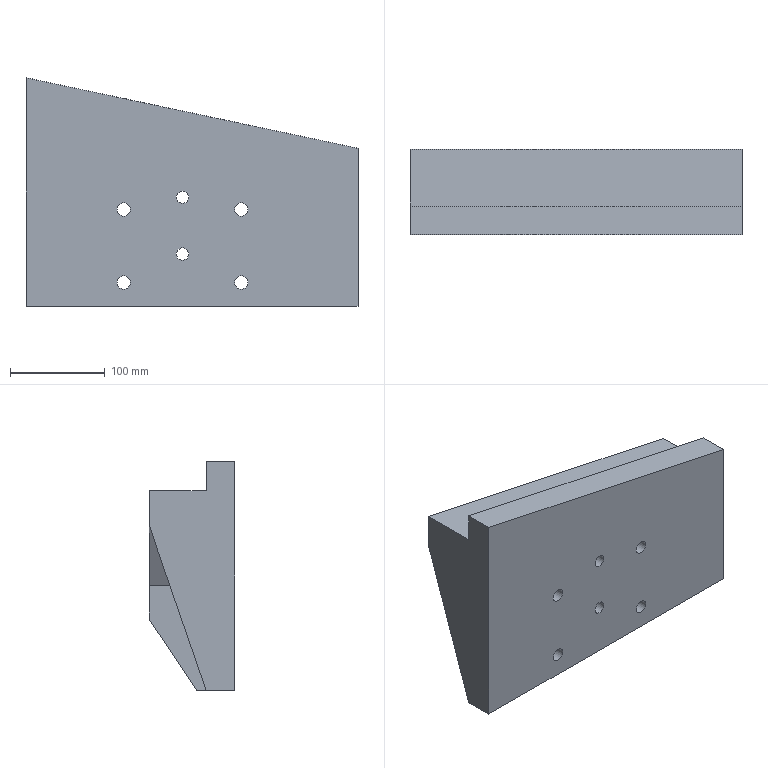Part | NX | features solid 2 | 1 solid | 28 faces | box 350 x 90 x 240.969 mm | volume 3053281 mm3 | plane 18 | cylinder 10 | commonest cylinder face diameters 14 x4 20 x4 13 x2
STEP:
#1=CARTESIAN_POINT('',(-565.,-580.,-83.));
#2=VERTEX_POINT('',#1);
#3=CARTESIAN_POINT('',(-572.,-580.,-83.));
#4=DIRECTION('',(0.,-1.,0.));
#5=DIRECTION('',(1.,0.,0.));
#6=AXIS2_PLACEMENT_3D('',#3,#4,#5);
#7=CIRCLE('',#6,7.);
#8=EDGE_CURVE('',#2,#2,#7,.T.);
#9=ORIENTED_EDGE('',*,*,#8,.T.);
#10=EDGE_LOOP('',(#9));
#11=FACE_BOUND('',#10,.T.);
#12=CARTESIAN_POINT('',(-562.,-580.,-83.));
#13=VERTEX_POINT('',#12);
#14=CARTESIAN_POINT('',(-572.,-580.,-83.));
#15=DIRECTION('',(0.,-1.,0.));
#16=DIRECTION('',(1.,0.,0.));
#17=AXIS2_PLACEMENT_3D('',#14,#15,#16);
#18=CIRCLE('',#17,10.);
#19=EDGE_CURVE('',#13,#13,#18,.T.);
#20=ORIENTED_EDGE('',*,*,#19,.F.);
#21=EDGE_LOOP('',(#20));
#22=FACE_BOUND('',#21,.T.);
#23=CARTESIAN_POINT('',(-572.,-580.,-83.));
#24=DIRECTION('',(0.,-1.,0.));
#25=DIRECTION('',(1.,0.,0.));
#26=AXIS2_PLACEMENT_3D('',#23,#24,#25);
#27=PLANE('',#26);
#28=ADVANCED_FACE('',(#11,#22),#27,.F.);
#29=CARTESIAN_POINT('',(-565.,-580.,-160.));
#30=VERTEX_POINT('',#29);
#31=CARTESIAN_POINT('',(-572.,-580.,-160.));
#32=DIRECTION('',(0.,-1.,0.));
#33=DIRECTION('',(1.,0.,0.));
#34=AXIS2_PLACEMENT_3D('',#31,#32,#33);
#35=CIRCLE('',#34,7.);
#36=EDGE_CURVE('',#30,#30,#35,.T.);
#37=ORIENTED_EDGE('',*,*,#36,.T.);
#38=EDGE_LOOP('',(#37));
#39=FACE_BOUND('',#38,.T.);
#40=CARTESIAN_POINT('',(-562.,-580.,-160.));
#41=VERTEX_POINT('',#40);
#42=CARTESIAN_POINT('',(-572.,-580.,-160.));
#43=DIRECTION('',(0.,-1.,0.));
#44=DIRECTION('',(1.,0.,0.));
#45=AXIS2_PLACEMENT_3D('',#42,#43,#44);
#46=CIRCLE('',#45,10.);
#47=EDGE_CURVE('',#41,#41,#46,.T.);
#48=ORIENTED_EDGE('',*,*,#47,.F.);
#49=EDGE_LOOP('',(#48));
#50=FACE_BOUND('',#49,.T.);
#51=CARTESIAN_POINT('',(-572.,-580.,-160.));
#52=DIRECTION('',(0.,-1.,0.));
#53=DIRECTION('',(1.,0.,0.));
#54=AXIS2_PLACEMENT_3D('',#51,#52,#53);
#55=PLANE('',#54);
#56=ADVANCED_FACE('',(#39,#50),#55,.F.);
#57=CARTESIAN_POINT('',(-441.,-580.,-160.));
#58=VERTEX_POINT('',#57);
#59=CARTESIAN_POINT('',(-448.,-580.,-160.));
#60=DIRECTION('',(0.,-1.,0.));
#61=DIRECTION('',(1.,0.,0.));
#62=AXIS2_PLACEMENT_3D('',#59,#60,#61);
#63=CIRCLE('',#62,7.);
#64=EDGE_CURVE('',#58,#58,#63,.T.);
#65=ORIENTED_EDGE('',*,*,#64,.T.);
#66=EDGE_LOOP('',(#65));
#67=FACE_BOUND('',#66,.T.);
#68=CARTESIAN_POINT('',(-438.,-580.,-160.));
#69=VERTEX_POINT('',#68);
#70=CARTESIAN_POINT('',(-448.,-580.,-160.));
#71=DIRECTION('',(0.,-1.,0.));
#72=DIRECTION('',(1.,0.,0.));
#73=AXIS2_PLACEMENT_3D('',#70,#71,#72);
#74=CIRCLE('',#73,10.);
#75=EDGE_CURVE('',#69,#69,#74,.T.);
#76=ORIENTED_EDGE('',*,*,#75,.F.);
#77=EDGE_LOOP('',(#76));
#78=FACE_BOUND('',#77,.T.);
#79=CARTESIAN_POINT('',(-448.,-580.,-160.));
#80=DIRECTION('',(0.,-1.,0.));
#81=DIRECTION('',(1.,0.,0.));
#82=AXIS2_PLACEMENT_3D('',#79,#80,#81);
#83=PLANE('',#82);
#84=ADVANCED_FACE('',(#67,#78),#83,.F.);
#85=CARTESIAN_POINT('',(-441.,-580.,-83.));
#86=VERTEX_POINT('',#85);
#87=CARTESIAN_POINT('',(-448.,-580.,-83.));
#88=DIRECTION('',(0.,-1.,0.));
#89=DIRECTION('',(1.,0.,0.));
#90=AXIS2_PLACEMENT_3D('',#87,#88,#89);
#91=CIRCLE('',#90,7.);
#92=EDGE_CURVE('',#86,#86,#91,.T.);
#93=ORIENTED_EDGE('',*,*,#92,.T.);
#94=EDGE_LOOP('',(#93));
#95=FACE_BOUND('',#94,.T.);
#96=CARTESIAN_POINT('',(-438.,-580.,-83.));
#97=VERTEX_POINT('',#96);
#98=CARTESIAN_POINT('',(-448.,-580.,-83.));
#99=DIRECTION('',(0.,-1.,0.));
#100=DIRECTION('',(1.,0.,0.));
#101=AXIS2_PLACEMENT_3D('',#98,#99,#100);
#102=CIRCLE('',#101,10.);
#103=EDGE_CURVE('',#97,#97,#102,.T.);
#104=ORIENTED_EDGE('',*,*,#103,.F.);
#105=EDGE_LOOP('',(#104));
#106=FACE_BOUND('',#105,.T.);
#107=CARTESIAN_POINT('',(-448.,-580.,-83.));
#108=DIRECTION('',(0.,-1.,0.));
#109=DIRECTION('',(1.,0.,0.));
#110=AXIS2_PLACEMENT_3D('',#107,#108,#109);
#111=PLANE('',#110);
#112=ADVANCED_FACE('',(#95,#106),#111,.F.);
#113=CARTESIAN_POINT('',(-640.,-570.,-12.811));
#114=VERTEX_POINT('',#113);
#115=CARTESIAN_POINT('',(-640.,-570.,-185.));
#116=VERTEX_POINT('',#115);
#117=CARTESIAN_POINT('',(-640.,-570.,-55.974));
#118=DIRECTION('',(0.,0.,-1.));
#119=VECTOR('',#118,1000.);
#120=LINE('',#117,#119);
#121=EDGE_CURVE('',#114,#116,#120,.T.);
#122=ORIENTED_EDGE('',*,*,#121,.T.);
#123=CARTESIAN_POINT('',(-640.,-510.368,-12.811));
#124=VERTEX_POINT('',#123);
#125=CARTESIAN_POINT('',(-640.,-551.446,-131.426));
#126=DIRECTION('',(0.,0.3272,0.9449));
#127=VECTOR('',#126,1000.);
#128=LINE('',#125,#127);
#129=EDGE_CURVE('',#116,#124,#128,.T.);
#130=ORIENTED_EDGE('',*,*,#129,.T.);
#131=CARTESIAN_POINT('',(-640.,-570.,-12.811));
#132=DIRECTION('',(0.,1.,0.));
#133=VECTOR('',#132,1000.);
#134=LINE('',#131,#133);
#135=EDGE_CURVE('',#114,#124,#134,.T.);
#136=ORIENTED_EDGE('',*,*,#135,.F.);
#137=EDGE_LOOP('',(#122,#130,#136));
#138=FACE_BOUND('',#137,.T.);
#139=CARTESIAN_POINT('',(-640.,-570.,-125.));
#140=DIRECTION('',(-1.,0.,0.));
#141=DIRECTION('',(0.,0.,-1.));
#142=AXIS2_PLACEMENT_3D('',#139,#140,#141);
#143=PLANE('',#142);
#144=ADVANCED_FACE('',(#138),#143,.F.);
#145=ORIENTED_EDGE('',*,*,#47,.T.);
#146=EDGE_LOOP('',(#145));
#147=FACE_BOUND('',#146,.T.);
#148=CARTESIAN_POINT('',(-562.,-570.,-160.));
#149=VERTEX_POINT('',#148);
#150=CARTESIAN_POINT('',(-572.,-570.,-160.));
#151=DIRECTION('',(0.,-1.,0.));
#152=DIRECTION('',(1.,0.,0.));
#153=AXIS2_PLACEMENT_3D('',#150,#151,#152);
#154=CIRCLE('',#153,10.);
#155=EDGE_CURVE('',#149,#149,#154,.T.);
#156=ORIENTED_EDGE('',*,*,#155,.F.);
#157=EDGE_LOOP('',(#156));
#158=FACE_BOUND('',#157,.T.);
#159=CARTESIAN_POINT('',(-572.,-570.,-160.));
#160=DIRECTION('',(0.,-1.,0.));
#161=DIRECTION('',(1.,0.,0.));
#162=AXIS2_PLACEMENT_3D('',#159,#160,#161);
#163=CYLINDRICAL_SURFACE('',#162,10.);
#164=ADVANCED_FACE('',(#147,#158),#163,.F.);
#165=ORIENTED_EDGE('',*,*,#75,.T.);
#166=EDGE_LOOP('',(#165));
#167=FACE_BOUND('',#166,.T.);
#168=CARTESIAN_POINT('',(-438.,-570.,-160.));
#169=VERTEX_POINT('',#168);
#170=CARTESIAN_POINT('',(-448.,-570.,-160.));
#171=DIRECTION('',(0.,-1.,0.));
#172=DIRECTION('',(1.,0.,0.));
#173=AXIS2_PLACEMENT_3D('',#170,#171,#172);
#174=CIRCLE('',#173,10.);
#175=EDGE_CURVE('',#169,#169,#174,.T.);
#176=ORIENTED_EDGE('',*,*,#175,.F.);
#177=EDGE_LOOP('',(#176));
#178=FACE_BOUND('',#177,.T.);
#179=CARTESIAN_POINT('',(-448.,-570.,-160.));
#180=DIRECTION('',(0.,-1.,0.));
#181=DIRECTION('',(1.,0.,0.));
#182=AXIS2_PLACEMENT_3D('',#179,#180,#181);
#183=CYLINDRICAL_SURFACE('',#182,10.);
#184=ADVANCED_FACE('',(#167,#178),#183,.F.);
#185=ORIENTED_EDGE('',*,*,#19,.T.);
#186=EDGE_LOOP('',(#185));
#187=FACE_BOUND('',#186,.T.);
#188=CARTESIAN_POINT('',(-562.,-570.,-83.));
#189=VERTEX_POINT('',#188);
#190=CARTESIAN_POINT('',(-572.,-570.,-83.));
#191=DIRECTION('',(0.,-1.,0.));
#192=DIRECTION('',(1.,0.,0.));
#193=AXIS2_PLACEMENT_3D('',#190,#191,#192);
#194=CIRCLE('',#193,10.);
#195=EDGE_CURVE('',#189,#189,#194,.T.);
#196=ORIENTED_EDGE('',*,*,#195,.F.);
#197=EDGE_LOOP('',(#196));
#198=FACE_BOUND('',#197,.T.);
#199=CARTESIAN_POINT('',(-572.,-570.,-83.));
#200=DIRECTION('',(0.,-1.,0.));
#201=DIRECTION('',(1.,0.,0.));
#202=AXIS2_PLACEMENT_3D('',#199,#200,#201);
#203=CYLINDRICAL_SURFACE('',#202,10.);
#204=ADVANCED_FACE('',(#187,#198),#203,.F.);
#205=ORIENTED_EDGE('',*,*,#103,.T.);
#206=EDGE_LOOP('',(#205));
#207=FACE_BOUND('',#206,.T.);
#208=CARTESIAN_POINT('',(-438.,-570.,-83.));
#209=VERTEX_POINT('',#208);
#210=CARTESIAN_POINT('',(-448.,-570.,-83.));
#211=DIRECTION('',(0.,-1.,0.));
#212=DIRECTION('',(1.,0.,0.));
#213=AXIS2_PLACEMENT_3D('',#210,#211,#212);
#214=CIRCLE('',#213,10.);
#215=EDGE_CURVE('',#209,#209,#214,.T.);
#216=ORIENTED_EDGE('',*,*,#215,.F.);
#217=EDGE_LOOP('',(#216));
#218=FACE_BOUND('',#217,.T.);
#219=CARTESIAN_POINT('',(-448.,-570.,-83.));
#220=DIRECTION('',(0.,-1.,0.));
#221=DIRECTION('',(1.,0.,0.));
#222=AXIS2_PLACEMENT_3D('',#219,#220,#221);
#223=CYLINDRICAL_SURFACE('',#222,10.);
#224=ADVANCED_FACE('',(#207,#218),#223,.F.);
#225=ORIENTED_EDGE('',*,*,#8,.F.);
#226=EDGE_LOOP('',(#225));
#227=FACE_BOUND('',#226,.T.);
#228=CARTESIAN_POINT('',(-565.,-600.,-83.));
#229=VERTEX_POINT('',#228);
#230=CARTESIAN_POINT('',(-572.,-600.,-83.));
#231=DIRECTION('',(0.,-1.,0.));
#232=DIRECTION('',(1.,0.,0.));
#233=AXIS2_PLACEMENT_3D('',#230,#231,#232);
#234=CIRCLE('',#233,7.);
#235=EDGE_CURVE('',#229,#229,#234,.F.);
#236=ORIENTED_EDGE('',*,*,#235,.F.);
#237=EDGE_LOOP('',(#236));
#238=FACE_BOUND('',#237,.T.);
#239=CARTESIAN_POINT('',(-572.,-700.,-83.));
#240=DIRECTION('',(0.,1.,0.));
#241=DIRECTION('',(0.,0.,-1.));
#242=AXIS2_PLACEMENT_3D('',#239,#240,#241);
#243=CYLINDRICAL_SURFACE('',#242,7.);
#244=ADVANCED_FACE('',(#227,#238),#243,.F.);
#245=CARTESIAN_POINT('',(-503.5,-600.,-70.));
#246=VERTEX_POINT('',#245);
#247=CARTESIAN_POINT('',(-510.,-600.,-70.));
#248=DIRECTION('',(0.,-1.,0.));
#249=DIRECTION('',(1.,0.,0.));
#250=AXIS2_PLACEMENT_3D('',#247,#248,#249);
#251=CIRCLE('',#250,6.5);
#252=EDGE_CURVE('',#246,#246,#251,.T.);
#253=ORIENTED_EDGE('',*,*,#252,.T.);
#254=EDGE_LOOP('',(#253));
#255=FACE_BOUND('',#254,.T.);
#256=CARTESIAN_POINT('',(-503.5,-570.,-70.));
#257=VERTEX_POINT('',#256);
#258=CARTESIAN_POINT('',(-510.,-570.,-70.));
#259=DIRECTION('',(0.,-1.,0.));
#260=DIRECTION('',(1.,0.,0.));
#261=AXIS2_PLACEMENT_3D('',#258,#259,#260);
#262=CIRCLE('',#261,6.5);
#263=EDGE_CURVE('',#257,#257,#262,.T.);
#264=ORIENTED_EDGE('',*,*,#263,.F.);
#265=EDGE_LOOP('',(#264));
#266=FACE_BOUND('',#265,.T.);
#267=CARTESIAN_POINT('',(-510.,-700.,-70.));
#268=DIRECTION('',(0.,1.,0.));
#269=DIRECTION('',(0.,0.,-1.));
#270=AXIS2_PLACEMENT_3D('',#267,#268,#269);
#271=CYLINDRICAL_SURFACE('',#270,6.5);
#272=ADVANCED_FACE('',(#255,#266),#271,.F.);
#273=ORIENTED_EDGE('',*,*,#36,.F.);
#274=EDGE_LOOP('',(#273));
#275=FACE_BOUND('',#274,.T.);
#276=CARTESIAN_POINT('',(-565.,-600.,-160.));
#277=VERTEX_POINT('',#276);
#278=CARTESIAN_POINT('',(-572.,-600.,-160.));
#279=DIRECTION('',(0.,-1.,0.));
#280=DIRECTION('',(1.,0.,0.));
#281=AXIS2_PLACEMENT_3D('',#278,#279,#280);
#282=CIRCLE('',#281,7.);
#283=EDGE_CURVE('',#277,#277,#282,.F.);
#284=ORIENTED_EDGE('',*,*,#283,.F.);
#285=EDGE_LOOP('',(#284));
#286=FACE_BOUND('',#285,.T.);
#287=CARTESIAN_POINT('',(-572.,-700.,-160.));
#288=DIRECTION('',(0.,1.,0.));
#289=DIRECTION('',(0.,0.,-1.));
#290=AXIS2_PLACEMENT_3D('',#287,#288,#289);
#291=CYLINDRICAL_SURFACE('',#290,7.);
#292=ADVANCED_FACE('',(#275,#286),#291,.F.);
#293=CARTESIAN_POINT('',(-503.5,-600.,-130.));
#294=VERTEX_POINT('',#293);
#295=CARTESIAN_POINT('',(-510.,-600.,-130.));
#296=DIRECTION('',(0.,-1.,0.));
#297=DIRECTION('',(1.,0.,0.));
#298=AXIS2_PLACEMENT_3D('',#295,#296,#297);
#299=CIRCLE('',#298,6.5);
#300=EDGE_CURVE('',#294,#294,#299,.T.);
#301=ORIENTED_EDGE('',*,*,#300,.T.);
#302=EDGE_LOOP('',(#301));
#303=FACE_BOUND('',#302,.T.);
#304=CARTESIAN_POINT('',(-503.5,-570.,-130.));
#305=VERTEX_POINT('',#304);
#306=CARTESIAN_POINT('',(-510.,-570.,-130.));
#307=DIRECTION('',(0.,-1.,0.));
#308=DIRECTION('',(1.,0.,0.));
#309=AXIS2_PLACEMENT_3D('',#306,#307,#308);
#310=CIRCLE('',#309,6.5);
#311=EDGE_CURVE('',#305,#305,#310,.T.);
#312=ORIENTED_EDGE('',*,*,#311,.F.);
#313=EDGE_LOOP('',(#312));
#314=FACE_BOUND('',#313,.T.);
#315=CARTESIAN_POINT('',(-510.,-700.,-130.));
#316=DIRECTION('',(0.,1.,0.));
#317=DIRECTION('',(0.,0.,-1.));
#318=AXIS2_PLACEMENT_3D('',#315,#316,#317);
#319=CYLINDRICAL_SURFACE('',#318,6.5);
#320=ADVANCED_FACE('',(#303,#314),#319,.F.);
#321=ORIENTED_EDGE('',*,*,#64,.F.);
#322=EDGE_LOOP('',(#321));
#323=FACE_BOUND('',#322,.T.);
#324=CARTESIAN_POINT('',(-441.,-600.,-160.));
#325=VERTEX_POINT('',#324);
#326=CARTESIAN_POINT('',(-448.,-600.,-160.));
#327=DIRECTION('',(0.,-1.,0.));
#328=DIRECTION('',(1.,0.,0.));
#329=AXIS2_PLACEMENT_3D('',#326,#327,#328);
#330=CIRCLE('',#329,7.);
#331=EDGE_CURVE('',#325,#325,#330,.F.);
#332=ORIENTED_EDGE('',*,*,#331,.F.);
#333=EDGE_LOOP('',(#332));
#334=FACE_BOUND('',#333,.T.);
#335=CARTESIAN_POINT('',(-448.,-700.,-160.));
#336=DIRECTION('',(0.,1.,0.));
#337=DIRECTION('',(0.,0.,-1.));
#338=AXIS2_PLACEMENT_3D('',#335,#336,#337);
#339=CYLINDRICAL_SURFACE('',#338,7.);
#340=ADVANCED_FACE('',(#323,#334),#339,.F.);
#341=ORIENTED_EDGE('',*,*,#92,.F.);
#342=EDGE_LOOP('',(#341));
#343=FACE_BOUND('',#342,.T.);
#344=CARTESIAN_POINT('',(-441.,-600.,-83.));
#345=VERTEX_POINT('',#344);
#346=CARTESIAN_POINT('',(-448.,-600.,-83.));
#347=DIRECTION('',(0.,-1.,0.));
#348=DIRECTION('',(1.,0.,0.));
#349=AXIS2_PLACEMENT_3D('',#346,#347,#348);
#350=CIRCLE('',#349,7.);
#351=EDGE_CURVE('',#345,#345,#350,.F.);
#352=ORIENTED_EDGE('',*,*,#351,.F.);
#353=EDGE_LOOP('',(#352));
#354=FACE_BOUND('',#353,.T.);
#355=CARTESIAN_POINT('',(-448.,-700.,-83.));
#356=DIRECTION('',(0.,1.,0.));
#357=DIRECTION('',(0.,0.,-1.));
#358=AXIS2_PLACEMENT_3D('',#355,#356,#357);
#359=CYLINDRICAL_SURFACE('',#358,7.);
#360=ADVANCED_FACE('',(#343,#354),#359,.F.);
#361=CARTESIAN_POINT('',(-675.,-600.,-185.));
#362=VERTEX_POINT('',#361);
#363=CARTESIAN_POINT('',(-675.,-570.,-185.));
#364=VERTEX_POINT('',#363);
#365=CARTESIAN_POINT('',(-675.,-600.,-185.));
#366=DIRECTION('',(0.,1.,0.));
#367=VECTOR('',#366,1000.);
#368=LINE('',#365,#367);
#369=EDGE_CURVE('',#362,#364,#368,.T.);
#370=ORIENTED_EDGE('',*,*,#369,.T.);
#371=CARTESIAN_POINT('',(-305.,-570.,-185.));
#372=DIRECTION('',(-1.,0.,0.));
#373=VECTOR('',#372,1000.);
#374=LINE('',#371,#373);
#375=EDGE_CURVE('',#116,#364,#374,.T.);
#376=ORIENTED_EDGE('',*,*,#375,.F.);
#377=CARTESIAN_POINT('',(-350.,-570.,-185.));
#378=VERTEX_POINT('',#377);
#379=CARTESIAN_POINT('',(-695.,-570.,-185.));
#380=DIRECTION('',(1.,0.,0.));
#381=VECTOR('',#380,1000.);
#382=LINE('',#379,#381);
#383=EDGE_CURVE('',#378,#116,#382,.F.);
#384=ORIENTED_EDGE('',*,*,#383,.F.);
#385=CARTESIAN_POINT('',(-350.,-560.,-185.));
#386=VERTEX_POINT('',#385);
#387=CARTESIAN_POINT('',(-350.,-570.,-185.));
#388=DIRECTION('',(0.,1.,0.));
#389=VECTOR('',#388,1000.);
#390=LINE('',#387,#389);
#391=EDGE_CURVE('',#386,#378,#390,.F.);
#392=ORIENTED_EDGE('',*,*,#391,.F.);
#393=CARTESIAN_POINT('',(-325.,-560.,-185.));
#394=VERTEX_POINT('',#393);
#395=CARTESIAN_POINT('',(-270.,-560.,-185.));
#396=DIRECTION('',(1.,0.,0.));
#397=VECTOR('',#396,1000.);
#398=LINE('',#395,#397);
#399=EDGE_CURVE('',#386,#394,#398,.T.);
#400=ORIENTED_EDGE('',*,*,#399,.T.);
#401=CARTESIAN_POINT('',(-325.,-600.,-185.));
#402=VERTEX_POINT('',#401);
#403=CARTESIAN_POINT('',(-325.,-515.,-185.));
#404=DIRECTION('',(0.,-1.,0.));
#405=VECTOR('',#404,1000.);
#406=LINE('',#403,#405);
#407=EDGE_CURVE('',#402,#394,#406,.F.);
#408=ORIENTED_EDGE('',*,*,#407,.F.);
#409=CARTESIAN_POINT('',(275.,-600.,-185.));
#410=DIRECTION('',(1.,0.,0.));
#411=VECTOR('',#410,1000.);
#412=LINE('',#409,#411);
#413=EDGE_CURVE('',#402,#362,#412,.F.);
#414=ORIENTED_EDGE('',*,*,#413,.T.);
#415=EDGE_LOOP('',(#370,#376,#384,#392,#400,#408,#414));
#416=FACE_BOUND('',#415,.T.);
#417=CARTESIAN_POINT('',(460.,-600.,-185.));
#418=DIRECTION('',(0.,0.,-1.));
#419=DIRECTION('',(0.,-1.,0.));
#420=AXIS2_PLACEMENT_3D('',#417,#418,#419);
#421=PLANE('',#420);
#422=ADVANCED_FACE('',(#416),#421,.T.);
#423=CARTESIAN_POINT('',(-675.,-570.,25.298));
#424=VERTEX_POINT('',#423);
#425=CARTESIAN_POINT('',(-675.,-570.,55.969));
#426=VERTEX_POINT('',#425);
#427=CARTESIAN_POINT('',(-675.,-570.,-55.974));
#428=DIRECTION('',(0.,0.,1.));
#429=VECTOR('',#428,1000.);
#430=LINE('',#427,#429);
#431=EDGE_CURVE('',#424,#426,#430,.T.);
#432=ORIENTED_EDGE('',*,*,#431,.F.);
#433=CARTESIAN_POINT('',(-675.,-510.,25.298));
#434=VERTEX_POINT('',#433);
#435=CARTESIAN_POINT('',(-675.,-5.,25.298));
#436=DIRECTION('',(0.,-1.,0.));
#437=VECTOR('',#436,1000.);
#438=LINE('',#435,#437);
#439=EDGE_CURVE('',#434,#424,#438,.T.);
#440=ORIENTED_EDGE('',*,*,#439,.F.);
#441=CARTESIAN_POINT('',(-675.,-510.,-11.749));
#442=VERTEX_POINT('',#441);
#443=CARTESIAN_POINT('',(-675.,-510.,-95.974));
#444=DIRECTION('',(0.,0.,-1.));
#445=VECTOR('',#444,1000.);
#446=LINE('',#443,#445);
#447=EDGE_CURVE('',#442,#434,#446,.F.);
#448=ORIENTED_EDGE('',*,*,#447,.F.);
#449=CARTESIAN_POINT('',(-675.,-452.286,154.903));
#450=DIRECTION('',(0.,0.3272,0.9449));
#451=VECTOR('',#450,1000.);
#452=LINE('',#449,#451);
#453=EDGE_CURVE('',#442,#364,#452,.F.);
#454=ORIENTED_EDGE('',*,*,#453,.T.);
#455=ORIENTED_EDGE('',*,*,#369,.F.);
#456=CARTESIAN_POINT('',(-675.,-600.,55.969));
#457=VERTEX_POINT('',#456);
#458=CARTESIAN_POINT('',(-675.,-600.,-55.974));
#459=DIRECTION('',(0.,0.,1.));
#460=VECTOR('',#459,1000.);
#461=LINE('',#458,#460);
#462=EDGE_CURVE('',#362,#457,#461,.T.);
#463=ORIENTED_EDGE('',*,*,#462,.T.);
#464=CARTESIAN_POINT('',(-675.,-5.,55.969));
#465=DIRECTION('',(0.,-1.,0.));
#466=VECTOR('',#465,1000.);
#467=LINE('',#464,#466);
#468=EDGE_CURVE('',#426,#457,#467,.T.);
#469=ORIENTED_EDGE('',*,*,#468,.F.);
#470=EDGE_LOOP('',(#432,#440,#448,#454,#455,#463,#469));
#471=FACE_BOUND('',#470,.T.);
#472=CARTESIAN_POINT('',(-675.,-5.,0.));
#473=DIRECTION('',(-1.,0.,0.));
#474=DIRECTION('',(0.,0.,-1.));
#475=AXIS2_PLACEMENT_3D('',#472,#473,#474);
#476=PLANE('',#475);
#477=ADVANCED_FACE('',(#471),#476,.T.);
#478=ORIENTED_EDGE('',*,*,#375,.T.);
#479=ORIENTED_EDGE('',*,*,#453,.F.);
#480=CARTESIAN_POINT('',(-645.,-510.,-11.749));
#481=VERTEX_POINT('',#480);
#482=CARTESIAN_POINT('',(-595.,-510.,-11.749));
#483=DIRECTION('',(-1.,0.,0.));
#484=VECTOR('',#483,1000.);
#485=LINE('',#482,#484);
#486=EDGE_CURVE('',#481,#442,#485,.T.);
#487=ORIENTED_EDGE('',*,*,#486,.F.);
#488=CARTESIAN_POINT('',(-558.152,-516.393,-30.209));
#489=DIRECTION('',(-0.9756,0.07182,0.2074));
#490=VECTOR('',#489,1000.);
#491=LINE('',#488,#490);
#492=EDGE_CURVE('',#124,#481,#491,.T.);
#493=ORIENTED_EDGE('',*,*,#492,.F.);
#494=ORIENTED_EDGE('',*,*,#129,.F.);
#495=EDGE_LOOP('',(#478,#479,#487,#493,#494));
#496=FACE_BOUND('',#495,.T.);
#497=CARTESIAN_POINT('',(-595.,-570.,-185.));
#498=DIRECTION('',(0.,-0.9449,0.3272));
#499=DIRECTION('',(0.,-0.3272,-0.9449));
#500=AXIS2_PLACEMENT_3D('',#497,#498,#499);
#501=PLANE('',#500);
#502=ADVANCED_FACE('',(#496),#501,.F.);
#503=ORIENTED_EDGE('',*,*,#135,.T.);
#504=ORIENTED_EDGE('',*,*,#492,.T.);
#505=CARTESIAN_POINT('',(-350.,-510.,-74.453));
#506=VERTEX_POINT('',#505);
#507=CARTESIAN_POINT('',(252.36,-510.,-202.488));
#508=DIRECTION('',(-0.9781,0.,0.2079));
#509=VECTOR('',#508,1000.);
#510=LINE('',#507,#509);
#511=EDGE_CURVE('',#506,#481,#510,.T.);
#512=ORIENTED_EDGE('',*,*,#511,.F.);
#513=CARTESIAN_POINT('',(-350.,-570.,-74.453));
#514=VERTEX_POINT('',#513);
#515=CARTESIAN_POINT('',(-350.,-570.,-74.453));
#516=DIRECTION('',(0.,-1.,0.));
#517=VECTOR('',#516,1000.);
#518=LINE('',#515,#517);
#519=EDGE_CURVE('',#514,#506,#518,.F.);
#520=ORIENTED_EDGE('',*,*,#519,.F.);
#521=CARTESIAN_POINT('',(-683.845,-570.,-3.492));
#522=DIRECTION('',(-0.9781,0.,0.2079));
#523=VECTOR('',#522,1000.);
#524=LINE('',#521,#523);
#525=EDGE_CURVE('',#514,#114,#524,.T.);
#526=ORIENTED_EDGE('',*,*,#525,.T.);
#527=EDGE_LOOP('',(#503,#504,#512,#520,#526));
#528=FACE_BOUND('',#527,.T.);
#529=CARTESIAN_POINT('',(-342.997,-570.,-75.941));
#530=DIRECTION('',(0.2079,0.,0.9781));
#531=DIRECTION('',(-0.9781,0.,0.2079));
#532=AXIS2_PLACEMENT_3D('',#529,#530,#531);
#533=PLANE('',#532);
#534=ADVANCED_FACE('',(#528),#533,.F.);
#535=CARTESIAN_POINT('',(-350.,-510.,-110.));
#536=VERTEX_POINT('',#535);
#537=CARTESIAN_POINT('',(-350.,-535.385,-148.077));
#538=DIRECTION('',(0.,-0.5547,-0.8321));
#539=VECTOR('',#538,1000.);
#540=LINE('',#537,#539);
#541=EDGE_CURVE('',#386,#536,#540,.F.);
#542=ORIENTED_EDGE('',*,*,#541,.F.);
#543=ORIENTED_EDGE('',*,*,#391,.T.);
#544=CARTESIAN_POINT('',(-350.,-570.,-125.));
#545=DIRECTION('',(0.,0.,1.));
#546=VECTOR('',#545,1000.);
#547=LINE('',#544,#546);
#548=EDGE_CURVE('',#514,#378,#547,.F.);
#549=ORIENTED_EDGE('',*,*,#548,.F.);
#550=ORIENTED_EDGE('',*,*,#519,.T.);
#551=CARTESIAN_POINT('',(-350.,-510.,-125.));
#552=DIRECTION('',(0.,0.,1.));
#553=VECTOR('',#552,1000.);
#554=LINE('',#551,#553);
#555=EDGE_CURVE('',#506,#536,#554,.F.);
#556=ORIENTED_EDGE('',*,*,#555,.T.);
#557=EDGE_LOOP('',(#542,#543,#549,#550,#556));
#558=FACE_BOUND('',#557,.T.);
#559=CARTESIAN_POINT('',(-350.,-570.,-125.));
#560=DIRECTION('',(-1.,0.,0.));
#561=DIRECTION('',(0.,0.,-1.));
#562=AXIS2_PLACEMENT_3D('',#559,#560,#561);
#563=PLANE('',#562);
#564=ADVANCED_FACE('',(#558),#563,.T.);
#565=CARTESIAN_POINT('',(-325.,-600.,-18.426));
#566=VERTEX_POINT('',#565);
#567=CARTESIAN_POINT('',(-325.,-600.,-55.974));
#568=DIRECTION('',(0.,0.,-1.));
#569=VECTOR('',#568,1000.);
#570=LINE('',#567,#569);
#571=EDGE_CURVE('',#566,#402,#570,.T.);
#572=ORIENTED_EDGE('',*,*,#571,.T.);
#573=ORIENTED_EDGE('',*,*,#407,.T.);
#574=CARTESIAN_POINT('',(-325.,-510.,-110.));
#575=VERTEX_POINT('',#574);
#576=CARTESIAN_POINT('',(-325.,-543.83,-160.745));
#577=DIRECTION('',(0.,0.5547,0.8321));
#578=VECTOR('',#577,1000.);
#579=LINE('',#576,#578);
#580=EDGE_CURVE('',#575,#394,#579,.F.);
#581=ORIENTED_EDGE('',*,*,#580,.F.);
#582=CARTESIAN_POINT('',(-325.,-510.,-49.096));
#583=VERTEX_POINT('',#582);
#584=CARTESIAN_POINT('',(-325.,-510.,-179.965));
#585=DIRECTION('',(0.,0.,-1.));
#586=VECTOR('',#585,1000.);
#587=LINE('',#584,#586);
#588=EDGE_CURVE('',#575,#583,#587,.F.);
#589=ORIENTED_EDGE('',*,*,#588,.T.);
#590=CARTESIAN_POINT('',(-325.,-570.,-49.096));
#591=VERTEX_POINT('',#590);
#592=CARTESIAN_POINT('',(-325.,-535.533,-49.096));
#593=DIRECTION('',(0.,-1.,0.));
#594=VECTOR('',#593,1000.);
#595=LINE('',#592,#594);
#596=EDGE_CURVE('',#583,#591,#595,.T.);
#597=ORIENTED_EDGE('',*,*,#596,.T.);
#598=CARTESIAN_POINT('',(-325.,-570.,-18.426));
#599=VERTEX_POINT('',#598);
#600=CARTESIAN_POINT('',(-325.,-570.,-90.));
#601=DIRECTION('',(0.,0.,1.));
#602=VECTOR('',#601,1000.);
#603=LINE('',#600,#602);
#604=EDGE_CURVE('',#591,#599,#603,.T.);
#605=ORIENTED_EDGE('',*,*,#604,.T.);
#606=CARTESIAN_POINT('',(-325.,-535.533,-18.426));
#607=DIRECTION('',(0.,-1.,0.));
#608=VECTOR('',#607,1000.);
#609=LINE('',#606,#608);
#610=EDGE_CURVE('',#599,#566,#609,.T.);
#611=ORIENTED_EDGE('',*,*,#610,.T.);
#612=EDGE_LOOP('',(#572,#573,#581,#589,#597,#605,#611));
#613=FACE_BOUND('',#612,.T.);
#614=CARTESIAN_POINT('',(-325.,-515.,-179.965));
#615=DIRECTION('',(1.,0.,0.));
#616=DIRECTION('',(0.,0.,-1.));
#617=AXIS2_PLACEMENT_3D('',#614,#615,#616);
#618=PLANE('',#617);
#619=ADVANCED_FACE('',(#613),#618,.T.);
#620=ORIENTED_EDGE('',*,*,#399,.F.);
#621=ORIENTED_EDGE('',*,*,#541,.T.);
#622=CARTESIAN_POINT('',(-270.,-510.,-110.));
#623=DIRECTION('',(-1.,0.,0.));
#624=VECTOR('',#623,1000.);
#625=LINE('',#622,#624);
#626=EDGE_CURVE('',#575,#536,#625,.T.);
#627=ORIENTED_EDGE('',*,*,#626,.F.);
#628=ORIENTED_EDGE('',*,*,#580,.T.);
#629=EDGE_LOOP('',(#620,#621,#627,#628));
#630=FACE_BOUND('',#629,.T.);
#631=CARTESIAN_POINT('',(-270.,-513.077,-114.615));
#632=DIRECTION('',(0.,0.8321,-0.5547));
#633=DIRECTION('',(0.,0.5547,0.8321));
#634=AXIS2_PLACEMENT_3D('',#631,#632,#633);
#635=PLANE('',#634);
#636=ADVANCED_FACE('',(#630),#635,.T.);
#637=CARTESIAN_POINT('',(256.7,-570.,-142.07));
#638=DIRECTION('',(0.9781,0.,-0.2079));
#639=VECTOR('',#638,1000.);
#640=LINE('',#637,#639);
#641=EDGE_CURVE('',#599,#426,#640,.F.);
#642=ORIENTED_EDGE('',*,*,#641,.F.);
#643=ORIENTED_EDGE('',*,*,#604,.F.);
#644=CARTESIAN_POINT('',(250.462,-570.,-171.415));
#645=DIRECTION('',(0.9781,0.,-0.2079));
#646=VECTOR('',#645,1000.);
#647=LINE('',#644,#646);
#648=EDGE_CURVE('',#591,#424,#647,.F.);
#649=ORIENTED_EDGE('',*,*,#648,.T.);
#650=ORIENTED_EDGE('',*,*,#431,.T.);
#651=EDGE_LOOP('',(#642,#643,#649,#650));
#652=FACE_BOUND('',#651,.T.);
#653=CARTESIAN_POINT('',(85.,-570.,-55.974));
#654=DIRECTION('',(0.,-1.,0.));
#655=DIRECTION('',(1.,0.,0.));
#656=AXIS2_PLACEMENT_3D('',#653,#654,#655);
#657=PLANE('',#656);
#658=ADVANCED_FACE('',(#652),#657,.F.);
#659=ORIENTED_EDGE('',*,*,#596,.F.);
#660=CARTESIAN_POINT('',(258.597,-510.,-173.144));
#661=DIRECTION('',(0.9781,0.,-0.2079));
#662=VECTOR('',#661,1000.);
#663=LINE('',#660,#662);
#664=EDGE_CURVE('',#583,#434,#663,.F.);
#665=ORIENTED_EDGE('',*,*,#664,.T.);
#666=ORIENTED_EDGE('',*,*,#439,.T.);
#667=ORIENTED_EDGE('',*,*,#648,.F.);
#668=EDGE_LOOP('',(#659,#665,#666,#667));
#669=FACE_BOUND('',#668,.T.);
#670=CARTESIAN_POINT('',(-493.346,-535.533,-13.313));
#671=DIRECTION('',(-0.2079,0.,-0.9781));
#672=DIRECTION('',(-0.9781,0.,0.2079));
#673=AXIS2_PLACEMENT_3D('',#670,#671,#672);
#674=PLANE('',#673);
#675=ADVANCED_FACE('',(#669),#674,.F.);
#676=ORIENTED_EDGE('',*,*,#588,.F.);
#677=ORIENTED_EDGE('',*,*,#626,.T.);
#678=ORIENTED_EDGE('',*,*,#555,.F.);
#679=ORIENTED_EDGE('',*,*,#511,.T.);
#680=ORIENTED_EDGE('',*,*,#486,.T.);
#681=ORIENTED_EDGE('',*,*,#447,.T.);
#682=ORIENTED_EDGE('',*,*,#664,.F.);
#683=EDGE_LOOP('',(#676,#677,#678,#679,#680,#681,#682));
#684=FACE_BOUND('',#683,.T.);
#685=CARTESIAN_POINT('',(275.,-510.,-95.974));
#686=DIRECTION('',(0.,-1.,0.));
#687=DIRECTION('',(1.,0.,0.));
#688=AXIS2_PLACEMENT_3D('',#685,#686,#687);
#689=PLANE('',#688);
#690=ADVANCED_FACE('',(#684),#689,.F.);
#691=CARTESIAN_POINT('',(256.7,-600.,-142.07));
#692=DIRECTION('',(0.9781,0.,-0.2079));
#693=VECTOR('',#692,1000.);
#694=LINE('',#691,#693);
#695=EDGE_CURVE('',#566,#457,#694,.F.);
#696=ORIENTED_EDGE('',*,*,#695,.F.);
#697=ORIENTED_EDGE('',*,*,#610,.F.);
#698=ORIENTED_EDGE('',*,*,#641,.T.);
#699=ORIENTED_EDGE('',*,*,#468,.T.);
#700=EDGE_LOOP('',(#696,#697,#698,#699));
#701=FACE_BOUND('',#700,.T.);
#702=CARTESIAN_POINT('',(-487.109,-535.533,16.031));
#703=DIRECTION('',(-0.2079,0.,-0.9781));
#704=DIRECTION('',(-0.9781,0.,0.2079));
#705=AXIS2_PLACEMENT_3D('',#702,#703,#704);
#706=PLANE('',#705);
#707=ADVANCED_FACE('',(#701),#706,.F.);
#708=ORIENTED_EDGE('',*,*,#413,.F.);
#709=ORIENTED_EDGE('',*,*,#571,.F.);
#710=ORIENTED_EDGE('',*,*,#695,.T.);
#711=ORIENTED_EDGE('',*,*,#462,.F.);
#712=EDGE_LOOP('',(#708,#709,#710,#711));
#713=FACE_BOUND('',#712,.T.);
#714=ORIENTED_EDGE('',*,*,#351,.T.);
#715=EDGE_LOOP('',(#714));
#716=FACE_BOUND('',#715,.T.);
#717=ORIENTED_EDGE('',*,*,#331,.T.);
#718=EDGE_LOOP('',(#717));
#719=FACE_BOUND('',#718,.T.);
#720=ORIENTED_EDGE('',*,*,#300,.F.);
#721=EDGE_LOOP('',(#720));
#722=FACE_BOUND('',#721,.T.);
#723=ORIENTED_EDGE('',*,*,#283,.T.);
#724=EDGE_LOOP('',(#723));
#725=FACE_BOUND('',#724,.T.);
#726=ORIENTED_EDGE('',*,*,#252,.F.);
#727=EDGE_LOOP('',(#726));
#728=FACE_BOUND('',#727,.T.);
#729=ORIENTED_EDGE('',*,*,#235,.T.);
#730=EDGE_LOOP('',(#729));
#731=FACE_BOUND('',#730,.T.);
#732=CARTESIAN_POINT('',(275.,-600.,-55.974));
#733=DIRECTION('',(0.,-1.,0.));
#734=DIRECTION('',(1.,0.,0.));
#735=AXIS2_PLACEMENT_3D('',#732,#733,#734);
#736=PLANE('',#735);
#737=ADVANCED_FACE('',(#713,#716,#719,#722,#725,#728,#731),#736,.T.);
#738=ORIENTED_EDGE('',*,*,#215,.T.);
#739=EDGE_LOOP('',(#738));
#740=FACE_BOUND('',#739,.T.);
#741=ORIENTED_EDGE('',*,*,#195,.T.);
#742=EDGE_LOOP('',(#741));
#743=FACE_BOUND('',#742,.T.);
#744=ORIENTED_EDGE('',*,*,#175,.T.);
#745=EDGE_LOOP('',(#744));
#746=FACE_BOUND('',#745,.T.);
#747=ORIENTED_EDGE('',*,*,#155,.T.);
#748=EDGE_LOOP('',(#747));
#749=FACE_BOUND('',#748,.T.);
#750=ORIENTED_EDGE('',*,*,#311,.T.);
#751=EDGE_LOOP('',(#750));
#752=FACE_BOUND('',#751,.T.);
#753=ORIENTED_EDGE('',*,*,#263,.T.);
#754=EDGE_LOOP('',(#753));
#755=FACE_BOUND('',#754,.T.);
#756=ORIENTED_EDGE('',*,*,#548,.T.);
#757=ORIENTED_EDGE('',*,*,#383,.T.);
#758=ORIENTED_EDGE('',*,*,#121,.F.);
#759=ORIENTED_EDGE('',*,*,#525,.F.);
#760=EDGE_LOOP('',(#756,#757,#758,#759));
#761=FACE_BOUND('',#760,.T.);
#762=CARTESIAN_POINT('',(85.,-570.,-55.974));
#763=DIRECTION('',(0.,-1.,0.));
#764=DIRECTION('',(1.,0.,0.));
#765=AXIS2_PLACEMENT_3D('',#762,#763,#764);
#766=PLANE('',#765);
#767=ADVANCED_FACE('',(#740,#743,#746,#749,#752,#755,#761),#766,.F.);
#768=CLOSED_SHELL('',(#28,#56,#84,#112,#144,#164,#184,#204,#224,#244,#272,#292,#320,#340,#360,#422,#477,#502,#534,#564,#619,#636,#658,#675,#690,#707,#737,#767));
#769=MANIFOLD_SOLID_BREP('',#768);
#770=(LENGTH_UNIT()NAMED_UNIT(*)SI_UNIT(.MILLI.,.METRE.));
#771=UNCERTAINTY_MEASURE_WITH_UNIT(LENGTH_MEASURE(0.00001),#770,'','');
#772=(NAMED_UNIT(*)PLANE_ANGLE_UNIT()SI_UNIT($,.RADIAN.));
#773=(NAMED_UNIT(*)SI_UNIT($,.STERADIAN.)SOLID_ANGLE_UNIT());
#774=(GEOMETRIC_REPRESENTATION_CONTEXT(3)GLOBAL_UNCERTAINTY_ASSIGNED_CONTEXT((#771))GLOBAL_UNIT_ASSIGNED_CONTEXT((#770,#772,#773))REPRESENTATION_CONTEXT('',''));
#775=ADVANCED_BREP_SHAPE_REPRESENTATION('',(#769),#774);